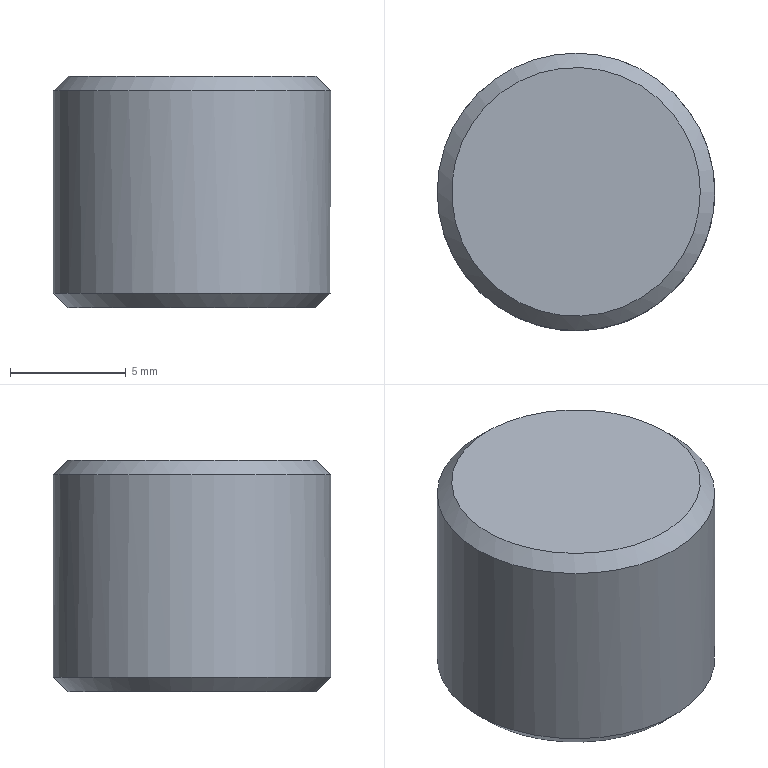Part | STEP file | MSW12-10_id1850_x_t | 1 solid | 5 faces | box 12.005 x 12.005 x 10 mm | volume 1118 mm3 | plane 2 | cone 2 | cylinder 1 | commonest cylinder face diameters 12.005 x1
STEP:
#1=CARTESIAN_POINT('',(336.623,-22.5,-95.));
#2=VERTEX_POINT('',#1);
#3=CARTESIAN_POINT('',(342.,-22.5,-95.));
#4=DIRECTION('',(0.,0.,-1.));
#5=DIRECTION('',(-1.,0.,0.));
#6=AXIS2_PLACEMENT_3D('',#3,#4,#5);
#7=CIRCLE('',#6,5.378);
#8=EDGE_CURVE('',#2,#2,#7,.T.);
#9=ORIENTED_EDGE('',*,*,#8,.T.);
#10=EDGE_LOOP('',(#9));
#11=FACE_OUTER_BOUND('',#10,.T.);
#12=CARTESIAN_POINT('',(342.,-22.5,-95.));
#13=DIRECTION('',(0.,0.,-1.));
#14=DIRECTION('',(-1.,0.,0.));
#15=AXIS2_PLACEMENT_3D('',#12,#13,#14);
#16=PLANE('',#15);
#17=ADVANCED_FACE('',(#11),#16,.T.);
#18=CARTESIAN_POINT('',(347.377,-22.5,-85.));
#19=VERTEX_POINT('',#18);
#20=CARTESIAN_POINT('',(342.,-22.5,-85.));
#21=DIRECTION('',(0.,0.,1.));
#22=DIRECTION('',(1.,0.,0.));
#23=AXIS2_PLACEMENT_3D('',#20,#21,#22);
#24=CIRCLE('',#23,5.378);
#25=EDGE_CURVE('',#19,#19,#24,.T.);
#26=ORIENTED_EDGE('',*,*,#25,.T.);
#27=EDGE_LOOP('',(#26));
#28=FACE_OUTER_BOUND('',#27,.T.);
#29=CARTESIAN_POINT('',(342.,-22.5,-85.));
#30=DIRECTION('',(0.,0.,1.));
#31=DIRECTION('',(1.,0.,0.));
#32=AXIS2_PLACEMENT_3D('',#29,#30,#31);
#33=PLANE('',#32);
#34=ADVANCED_FACE('',(#28),#33,.T.);
#35=CARTESIAN_POINT('',(348.002,-22.5,-85.625));
#36=VERTEX_POINT('',#35);
#37=CARTESIAN_POINT('',(342.,-22.5,-85.625));
#38=DIRECTION('',(0.,0.,-1.));
#39=DIRECTION('',(1.,0.,0.));
#40=AXIS2_PLACEMENT_3D('',#37,#38,#39);
#41=CIRCLE('',#40,6.003);
#42=EDGE_CURVE('',#36,#36,#41,.T.);
#43=ORIENTED_EDGE('',*,*,#42,.T.);
#44=EDGE_LOOP('',(#43));
#45=FACE_BOUND('',#44,.T.);
#46=CARTESIAN_POINT('',(335.998,-22.5,-94.375));
#47=VERTEX_POINT('',#46);
#48=CARTESIAN_POINT('',(342.,-22.5,-94.375));
#49=DIRECTION('',(0.,0.,1.));
#50=DIRECTION('',(-1.,0.,0.));
#51=AXIS2_PLACEMENT_3D('',#48,#49,#50);
#52=CIRCLE('',#51,6.003);
#53=EDGE_CURVE('',#47,#47,#52,.T.);
#54=ORIENTED_EDGE('',*,*,#53,.T.);
#55=EDGE_LOOP('',(#54));
#56=FACE_BOUND('',#55,.T.);
#57=CARTESIAN_POINT('',(342.,-22.5,-2.));
#58=DIRECTION('',(0.,0.,-1.));
#59=DIRECTION('',(-1.,0.,0.));
#60=AXIS2_PLACEMENT_3D('',#57,#58,#59);
#61=CYLINDRICAL_SURFACE('',#60,6.003);
#62=ADVANCED_FACE('',(#45,#56),#61,.T.);
#63=ORIENTED_EDGE('',*,*,#25,.F.);
#64=EDGE_LOOP('',(#63));
#65=FACE_BOUND('',#64,.T.);
#66=ORIENTED_EDGE('',*,*,#42,.F.);
#67=EDGE_LOOP('',(#66));
#68=FACE_BOUND('',#67,.T.);
#69=CARTESIAN_POINT('',(342.,-22.5,-85.625));
#70=DIRECTION('',(0.,0.,-1.));
#71=DIRECTION('',(-1.,0.,0.));
#72=AXIS2_PLACEMENT_3D('',#69,#70,#71);
#73=CONICAL_SURFACE('',#72,6.003,45.);
#74=ADVANCED_FACE('',(#65,#68),#73,.T.);
#75=ORIENTED_EDGE('',*,*,#8,.F.);
#76=EDGE_LOOP('',(#75));
#77=FACE_BOUND('',#76,.T.);
#78=ORIENTED_EDGE('',*,*,#53,.F.);
#79=EDGE_LOOP('',(#78));
#80=FACE_BOUND('',#79,.T.);
#81=CARTESIAN_POINT('',(342.,-22.5,-94.375));
#82=DIRECTION('',(0.,0.,1.));
#83=DIRECTION('',(1.,0.,0.));
#84=AXIS2_PLACEMENT_3D('',#81,#82,#83);
#85=CONICAL_SURFACE('',#84,6.003,45.);
#86=ADVANCED_FACE('',(#77,#80),#85,.T.);
#87=CLOSED_SHELL('',(#17,#34,#62,#74,#86));
#88=MANIFOLD_SOLID_BREP('',#87);
#89=(LENGTH_UNIT()NAMED_UNIT(*)SI_UNIT(.MILLI.,.METRE.));
#90=UNCERTAINTY_MEASURE_WITH_UNIT(LENGTH_MEASURE(0.00002),#89,'','');
#91=(NAMED_UNIT(*)PLANE_ANGLE_UNIT()SI_UNIT($,.RADIAN.));
#92=PLANE_ANGLE_MEASURE_WITH_UNIT(PLANE_ANGLE_MEASURE(0.01745),#91);
#93=DIMENSIONAL_EXPONENTS(0.,0.,0.,0.,0.,0.,0.);
#94=(CONVERSION_BASED_UNIT('DEGREE',#92)NAMED_UNIT(#93)PLANE_ANGLE_UNIT());
#95=(NAMED_UNIT(*)SI_UNIT($,.STERADIAN.)SOLID_ANGLE_UNIT());
#96=(GEOMETRIC_REPRESENTATION_CONTEXT(3)GLOBAL_UNCERTAINTY_ASSIGNED_CONTEXT((#90))GLOBAL_UNIT_ASSIGNED_CONTEXT((#89,#94,#95))REPRESENTATION_CONTEXT('',''));
#97=ADVANCED_BREP_SHAPE_REPRESENTATION('',(#88),#96);